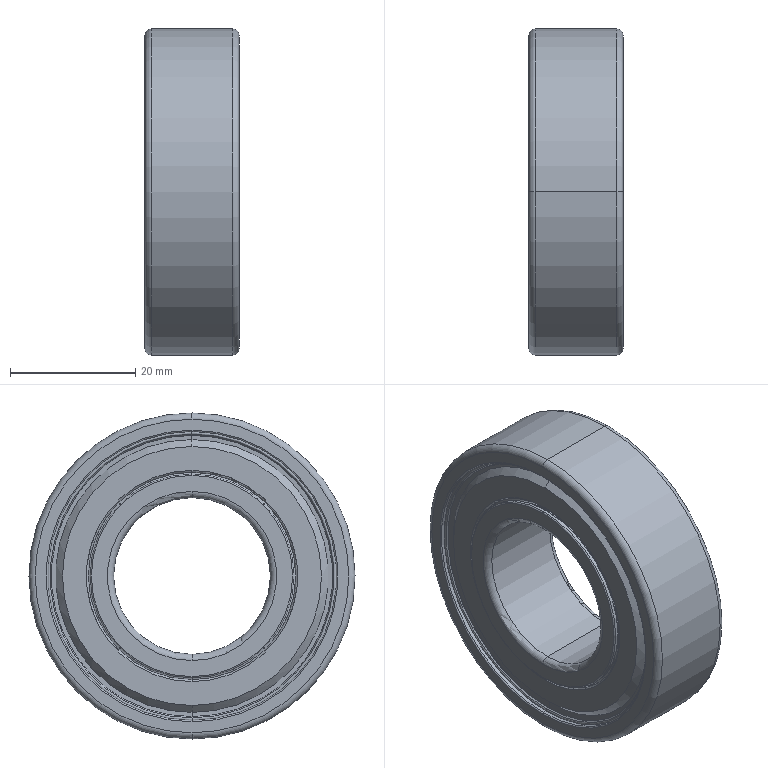Part | STEP file | HI_BAY6205ZZ^BFU71-6205ZZ-L55-S20_Mechanical tensioner (pay-off) | 1 solid | 136 faces | box 15 x 52 x 52 mm | volume 19388 mm3 | torus 56 | cone 40 | cylinder 28 | plane 12 | commonest cylinder face diameters 32.5 x4 33.1 x4 33.7 x4 34.1 x4 43.9 x4 25 x2